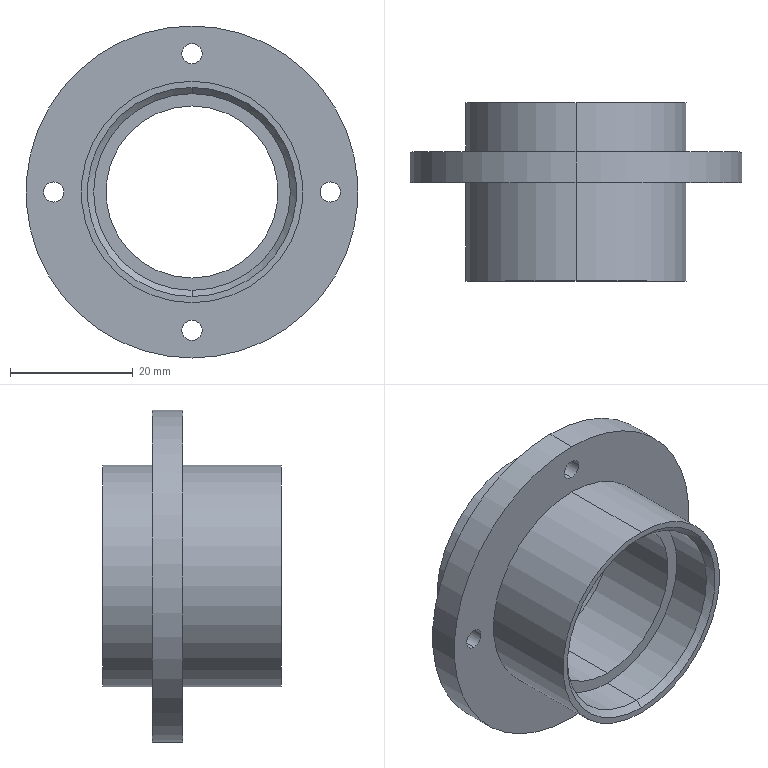Part | SolidWorks | features ICE 5, Chamfer 1, Extrusion 1, HoleWzd 1 | 1 solid | 30 faces | box 54 x 29 x 54 mm | volume 14771 mm3 | cylinder 20 | plane 6 | cone 4 | commonest cylinder face diameters 3.3 x8 32 x4 36 x4 28 x2 54 x2
STEP:
#1=CARTESIAN_POINT('',(0.,7.,-16.));
#2=VERTEX_POINT('',#1);
#3=CARTESIAN_POINT('',(0.,7.,16.));
#4=VERTEX_POINT('',#3);
#5=CARTESIAN_POINT('',(0.,7.,0.));
#6=DIRECTION('',(0.,1.,0.));
#7=DIRECTION('',(0.,0.,1.));
#8=AXIS2_PLACEMENT_3D('',#5,#6,#7);
#9=CIRCLE('',#8,16.);
#10=EDGE_CURVE('',#2,#4,#9,.T.);
#11=ORIENTED_EDGE('',*,*,#10,.F.);
#12=CARTESIAN_POINT('',(0.,8.,-17.));
#13=VERTEX_POINT('',#12);
#14=CARTESIAN_POINT('',(0.,8.,-17.));
#15=DIRECTION('',(0.,0.7071,-0.7071));
#16=VECTOR('',#15,1000.);
#17=LINE('',#14,#16);
#18=EDGE_CURVE('',#2,#13,#17,.T.);
#19=ORIENTED_EDGE('',*,*,#18,.T.);
#20=CARTESIAN_POINT('',(0.,8.,17.));
#21=VERTEX_POINT('',#20);
#22=CARTESIAN_POINT('',(0.,8.,0.));
#23=DIRECTION('',(0.,-1.,0.));
#24=DIRECTION('',(0.,0.,1.));
#25=AXIS2_PLACEMENT_3D('',#22,#23,#24);
#26=CIRCLE('',#25,17.);
#27=EDGE_CURVE('',#21,#13,#26,.T.);
#28=ORIENTED_EDGE('',*,*,#27,.F.);
#29=CARTESIAN_POINT('',(0.,8.,17.));
#30=DIRECTION('',(0.,0.7071,0.7071));
#31=VECTOR('',#30,1000.);
#32=LINE('',#29,#31);
#33=EDGE_CURVE('',#4,#21,#32,.T.);
#34=ORIENTED_EDGE('',*,*,#33,.F.);
#35=EDGE_LOOP('',(#11,#19,#28,#34));
#36=FACE_OUTER_BOUND('',#35,.T.);
#37=CARTESIAN_POINT('',(0.,8.,0.));
#38=DIRECTION('',(0.,1.,0.));
#39=DIRECTION('',(0.,0.,1.));
#40=AXIS2_PLACEMENT_3D('',#37,#38,#39);
#41=CONICAL_SURFACE('',#40,17.,0.7854);
#42=ADVANCED_FACE('',(#36),#41,.F.);
#43=CARTESIAN_POINT('',(0.,-20.,16.));
#44=VERTEX_POINT('',#43);
#45=CARTESIAN_POINT('',(0.,-20.,-16.));
#46=VERTEX_POINT('',#45);
#47=CARTESIAN_POINT('',(0.,-20.,0.));
#48=DIRECTION('',(0.,-1.,0.));
#49=DIRECTION('',(0.,0.,-1.));
#50=AXIS2_PLACEMENT_3D('',#47,#48,#49);
#51=CIRCLE('',#50,16.);
#52=EDGE_CURVE('',#44,#46,#51,.T.);
#53=ORIENTED_EDGE('',*,*,#52,.F.);
#54=CARTESIAN_POINT('',(0.,-21.,17.));
#55=VERTEX_POINT('',#54);
#56=CARTESIAN_POINT('',(0.,-20.,16.));
#57=DIRECTION('',(0.,-0.7071,0.7071));
#58=VECTOR('',#57,1000.);
#59=LINE('',#56,#58);
#60=EDGE_CURVE('',#44,#55,#59,.T.);
#61=ORIENTED_EDGE('',*,*,#60,.T.);
#62=CARTESIAN_POINT('',(0.,-21.,-17.));
#63=VERTEX_POINT('',#62);
#64=CARTESIAN_POINT('',(0.,-21.,0.));
#65=DIRECTION('',(0.,1.,0.));
#66=DIRECTION('',(0.,0.,-1.));
#67=AXIS2_PLACEMENT_3D('',#64,#65,#66);
#68=CIRCLE('',#67,17.);
#69=EDGE_CURVE('',#63,#55,#68,.T.);
#70=ORIENTED_EDGE('',*,*,#69,.F.);
#71=CARTESIAN_POINT('',(0.,-20.,-16.));
#72=DIRECTION('',(0.,-0.7071,-0.7071));
#73=VECTOR('',#72,1000.);
#74=LINE('',#71,#73);
#75=EDGE_CURVE('',#46,#63,#74,.T.);
#76=ORIENTED_EDGE('',*,*,#75,.F.);
#77=EDGE_LOOP('',(#53,#61,#70,#76));
#78=FACE_OUTER_BOUND('',#77,.T.);
#79=CARTESIAN_POINT('',(0.,-20.,0.));
#80=DIRECTION('',(0.,-1.,0.));
#81=DIRECTION('',(0.,0.,-1.));
#82=AXIS2_PLACEMENT_3D('',#79,#80,#81);
#83=CONICAL_SURFACE('',#82,16.,0.7854);
#84=ADVANCED_FACE('',(#78),#83,.F.);
#85=CARTESIAN_POINT('',(-22.5,-5.,1.65));
#86=VERTEX_POINT('',#85);
#87=CARTESIAN_POINT('',(-22.5,-5.,-1.65));
#88=VERTEX_POINT('',#87);
#89=CARTESIAN_POINT('',(-22.5,-5.,0.));
#90=DIRECTION('',(0.,-1.,0.));
#91=DIRECTION('',(0.,0.,-1.));
#92=AXIS2_PLACEMENT_3D('',#89,#90,#91);
#93=CIRCLE('',#92,1.65);
#94=EDGE_CURVE('',#86,#88,#93,.T.);
#95=ORIENTED_EDGE('',*,*,#94,.T.);
#96=CARTESIAN_POINT('',(-22.5,0.,-1.65));
#97=VERTEX_POINT('',#96);
#98=CARTESIAN_POINT('',(-22.5,0.,-1.65));
#99=DIRECTION('',(0.,1.,0.));
#100=VECTOR('',#99,1000.);
#101=LINE('',#98,#100);
#102=EDGE_CURVE('',#88,#97,#101,.T.);
#103=ORIENTED_EDGE('',*,*,#102,.T.);
#104=CARTESIAN_POINT('',(-22.5,0.,1.65));
#105=VERTEX_POINT('',#104);
#106=CARTESIAN_POINT('',(-22.5,0.,0.));
#107=DIRECTION('',(0.,1.,0.));
#108=DIRECTION('',(0.,0.,1.));
#109=AXIS2_PLACEMENT_3D('',#106,#107,#108);
#110=CIRCLE('',#109,1.65);
#111=EDGE_CURVE('',#97,#105,#110,.T.);
#112=ORIENTED_EDGE('',*,*,#111,.T.);
#113=CARTESIAN_POINT('',(-22.5,0.,1.65));
#114=DIRECTION('',(0.,1.,0.));
#115=VECTOR('',#114,1000.);
#116=LINE('',#113,#115);
#117=EDGE_CURVE('',#86,#105,#116,.T.);
#118=ORIENTED_EDGE('',*,*,#117,.F.);
#119=EDGE_LOOP('',(#95,#103,#112,#118));
#120=FACE_OUTER_BOUND('',#119,.T.);
#121=CARTESIAN_POINT('',(-22.5,0.,0.));
#122=DIRECTION('',(0.,1.,0.));
#123=DIRECTION('',(0.,0.,1.));
#124=AXIS2_PLACEMENT_3D('',#121,#122,#123);
#125=CYLINDRICAL_SURFACE('',#124,1.65);
#126=ADVANCED_FACE('',(#120),#125,.F.);
#127=CARTESIAN_POINT('',(0.,-5.,-20.85));
#128=VERTEX_POINT('',#127);
#129=CARTESIAN_POINT('',(0.,-5.,-24.15));
#130=VERTEX_POINT('',#129);
#131=CARTESIAN_POINT('',(0.,-5.,-22.5));
#132=DIRECTION('',(0.,-1.,0.));
#133=DIRECTION('',(0.,0.,-1.));
#134=AXIS2_PLACEMENT_3D('',#131,#132,#133);
#135=CIRCLE('',#134,1.65);
#136=EDGE_CURVE('',#128,#130,#135,.T.);
#137=ORIENTED_EDGE('',*,*,#136,.T.);
#138=CARTESIAN_POINT('',(0.,0.,-24.15));
#139=VERTEX_POINT('',#138);
#140=CARTESIAN_POINT('',(0.,0.,-24.15));
#141=DIRECTION('',(0.,1.,0.));
#142=VECTOR('',#141,1000.);
#143=LINE('',#140,#142);
#144=EDGE_CURVE('',#130,#139,#143,.T.);
#145=ORIENTED_EDGE('',*,*,#144,.T.);
#146=CARTESIAN_POINT('',(0.,0.,-20.85));
#147=VERTEX_POINT('',#146);
#148=CARTESIAN_POINT('',(0.,0.,-22.5));
#149=DIRECTION('',(0.,1.,0.));
#150=DIRECTION('',(0.,0.,1.));
#151=AXIS2_PLACEMENT_3D('',#148,#149,#150);
#152=CIRCLE('',#151,1.65);
#153=EDGE_CURVE('',#139,#147,#152,.T.);
#154=ORIENTED_EDGE('',*,*,#153,.T.);
#155=CARTESIAN_POINT('',(0.,0.,-20.85));
#156=DIRECTION('',(0.,1.,0.));
#157=VECTOR('',#156,1000.);
#158=LINE('',#155,#157);
#159=EDGE_CURVE('',#128,#147,#158,.T.);
#160=ORIENTED_EDGE('',*,*,#159,.F.);
#161=EDGE_LOOP('',(#137,#145,#154,#160));
#162=FACE_OUTER_BOUND('',#161,.T.);
#163=CARTESIAN_POINT('',(0.,0.,-22.5));
#164=DIRECTION('',(0.,1.,0.));
#165=DIRECTION('',(0.,0.,1.));
#166=AXIS2_PLACEMENT_3D('',#163,#164,#165);
#167=CYLINDRICAL_SURFACE('',#166,1.65);
#168=ADVANCED_FACE('',(#162),#167,.F.);
#169=CARTESIAN_POINT('',(22.5,-5.,1.65));
#170=VERTEX_POINT('',#169);
#171=CARTESIAN_POINT('',(22.5,-5.,-1.65));
#172=VERTEX_POINT('',#171);
#173=CARTESIAN_POINT('',(22.5,-5.,0.));
#174=DIRECTION('',(0.,-1.,0.));
#175=DIRECTION('',(0.,0.,-1.));
#176=AXIS2_PLACEMENT_3D('',#173,#174,#175);
#177=CIRCLE('',#176,1.65);
#178=EDGE_CURVE('',#170,#172,#177,.T.);
#179=ORIENTED_EDGE('',*,*,#178,.T.);
#180=CARTESIAN_POINT('',(22.5,0.,-1.65));
#181=VERTEX_POINT('',#180);
#182=CARTESIAN_POINT('',(22.5,0.,-1.65));
#183=DIRECTION('',(0.,1.,0.));
#184=VECTOR('',#183,1000.);
#185=LINE('',#182,#184);
#186=EDGE_CURVE('',#172,#181,#185,.T.);
#187=ORIENTED_EDGE('',*,*,#186,.T.);
#188=CARTESIAN_POINT('',(22.5,0.,1.65));
#189=VERTEX_POINT('',#188);
#190=CARTESIAN_POINT('',(22.5,0.,0.));
#191=DIRECTION('',(0.,1.,0.));
#192=DIRECTION('',(0.,0.,1.));
#193=AXIS2_PLACEMENT_3D('',#190,#191,#192);
#194=CIRCLE('',#193,1.65);
#195=EDGE_CURVE('',#181,#189,#194,.T.);
#196=ORIENTED_EDGE('',*,*,#195,.T.);
#197=CARTESIAN_POINT('',(22.5,0.,1.65));
#198=DIRECTION('',(0.,1.,0.));
#199=VECTOR('',#198,1000.);
#200=LINE('',#197,#199);
#201=EDGE_CURVE('',#170,#189,#200,.T.);
#202=ORIENTED_EDGE('',*,*,#201,.F.);
#203=EDGE_LOOP('',(#179,#187,#196,#202));
#204=FACE_OUTER_BOUND('',#203,.T.);
#205=CARTESIAN_POINT('',(22.5,0.,0.));
#206=DIRECTION('',(0.,1.,0.));
#207=DIRECTION('',(0.,0.,1.));
#208=AXIS2_PLACEMENT_3D('',#205,#206,#207);
#209=CYLINDRICAL_SURFACE('',#208,1.65);
#210=ADVANCED_FACE('',(#204),#209,.F.);
#211=CARTESIAN_POINT('',(0.,-5.,24.15));
#212=VERTEX_POINT('',#211);
#213=CARTESIAN_POINT('',(0.,-5.,20.85));
#214=VERTEX_POINT('',#213);
#215=CARTESIAN_POINT('',(0.,-5.,22.5));
#216=DIRECTION('',(0.,-1.,0.));
#217=DIRECTION('',(0.,0.,-1.));
#218=AXIS2_PLACEMENT_3D('',#215,#216,#217);
#219=CIRCLE('',#218,1.65);
#220=EDGE_CURVE('',#212,#214,#219,.T.);
#221=ORIENTED_EDGE('',*,*,#220,.T.);
#222=CARTESIAN_POINT('',(0.,0.,20.85));
#223=VERTEX_POINT('',#222);
#224=CARTESIAN_POINT('',(0.,0.,20.85));
#225=DIRECTION('',(0.,1.,0.));
#226=VECTOR('',#225,1000.);
#227=LINE('',#224,#226);
#228=EDGE_CURVE('',#214,#223,#227,.T.);
#229=ORIENTED_EDGE('',*,*,#228,.T.);
#230=CARTESIAN_POINT('',(0.,0.,24.15));
#231=VERTEX_POINT('',#230);
#232=CARTESIAN_POINT('',(0.,0.,22.5));
#233=DIRECTION('',(0.,1.,0.));
#234=DIRECTION('',(0.,0.,1.));
#235=AXIS2_PLACEMENT_3D('',#232,#233,#234);
#236=CIRCLE('',#235,1.65);
#237=EDGE_CURVE('',#223,#231,#236,.T.);
#238=ORIENTED_EDGE('',*,*,#237,.T.);
#239=CARTESIAN_POINT('',(0.,0.,24.15));
#240=DIRECTION('',(0.,1.,0.));
#241=VECTOR('',#240,1000.);
#242=LINE('',#239,#241);
#243=EDGE_CURVE('',#212,#231,#242,.T.);
#244=ORIENTED_EDGE('',*,*,#243,.F.);
#245=EDGE_LOOP('',(#221,#229,#238,#244));
#246=FACE_OUTER_BOUND('',#245,.T.);
#247=CARTESIAN_POINT('',(0.,0.,22.5));
#248=DIRECTION('',(0.,1.,0.));
#249=DIRECTION('',(0.,0.,1.));
#250=AXIS2_PLACEMENT_3D('',#247,#248,#249);
#251=CYLINDRICAL_SURFACE('',#250,1.65);
#252=ADVANCED_FACE('',(#246),#251,.F.);
#253=CARTESIAN_POINT('',(0.,-13.2,14.));
#254=VERTEX_POINT('',#253);
#255=CARTESIAN_POINT('',(0.,-13.2,-14.));
#256=VERTEX_POINT('',#255);
#257=CARTESIAN_POINT('',(0.,-13.2,0.));
#258=DIRECTION('',(0.,-1.,0.));
#259=DIRECTION('',(0.,0.,-1.));
#260=AXIS2_PLACEMENT_3D('',#257,#258,#259);
#261=CIRCLE('',#260,14.);
#262=EDGE_CURVE('',#254,#256,#261,.T.);
#263=ORIENTED_EDGE('',*,*,#262,.T.);
#264=CARTESIAN_POINT('',(0.,0.,-14.));
#265=VERTEX_POINT('',#264);
#266=CARTESIAN_POINT('',(0.,-21.,-14.));
#267=DIRECTION('',(0.,1.,0.));
#268=VECTOR('',#267,1000.);
#269=LINE('',#266,#268);
#270=EDGE_CURVE('',#256,#265,#269,.T.);
#271=ORIENTED_EDGE('',*,*,#270,.T.);
#272=CARTESIAN_POINT('',(0.,0.,14.));
#273=VERTEX_POINT('',#272);
#274=CARTESIAN_POINT('',(0.,0.,0.));
#275=DIRECTION('',(0.,1.,0.));
#276=DIRECTION('',(0.,0.,1.));
#277=AXIS2_PLACEMENT_3D('',#274,#275,#276);
#278=CIRCLE('',#277,14.);
#279=EDGE_CURVE('',#265,#273,#278,.T.);
#280=ORIENTED_EDGE('',*,*,#279,.T.);
#281=CARTESIAN_POINT('',(0.,-21.,14.));
#282=DIRECTION('',(0.,1.,0.));
#283=VECTOR('',#282,1000.);
#284=LINE('',#281,#283);
#285=EDGE_CURVE('',#254,#273,#284,.T.);
#286=ORIENTED_EDGE('',*,*,#285,.F.);
#287=EDGE_LOOP('',(#263,#271,#280,#286));
#288=FACE_OUTER_BOUND('',#287,.T.);
#289=CARTESIAN_POINT('',(0.,-21.,0.));
#290=DIRECTION('',(0.,1.,0.));
#291=DIRECTION('',(0.,0.,1.));
#292=AXIS2_PLACEMENT_3D('',#289,#290,#291);
#293=CYLINDRICAL_SURFACE('',#292,14.);
#294=ADVANCED_FACE('',(#288),#293,.F.);
#295=CARTESIAN_POINT('',(0.,-13.2,16.));
#296=VERTEX_POINT('',#295);
#297=CARTESIAN_POINT('',(0.,-13.2,-16.));
#298=VERTEX_POINT('',#297);
#299=CARTESIAN_POINT('',(0.,-13.2,0.));
#300=DIRECTION('',(0.,-1.,0.));
#301=DIRECTION('',(0.,0.,-1.));
#302=AXIS2_PLACEMENT_3D('',#299,#300,#301);
#303=CIRCLE('',#302,16.);
#304=EDGE_CURVE('',#296,#298,#303,.T.);
#305=ORIENTED_EDGE('',*,*,#304,.F.);
#306=CARTESIAN_POINT('',(0.,-13.2,16.));
#307=DIRECTION('',(0.,-1.,0.));
#308=VECTOR('',#307,1000.);
#309=LINE('',#306,#308);
#310=EDGE_CURVE('',#296,#44,#309,.T.);
#311=ORIENTED_EDGE('',*,*,#310,.T.);
#312=ORIENTED_EDGE('',*,*,#52,.T.);
#313=CARTESIAN_POINT('',(0.,-13.2,-16.));
#314=DIRECTION('',(0.,-1.,0.));
#315=VECTOR('',#314,1000.);
#316=LINE('',#313,#315);
#317=EDGE_CURVE('',#298,#46,#316,.T.);
#318=ORIENTED_EDGE('',*,*,#317,.F.);
#319=EDGE_LOOP('',(#305,#311,#312,#318));
#320=FACE_OUTER_BOUND('',#319,.T.);
#321=CARTESIAN_POINT('',(0.,-13.2,0.));
#322=DIRECTION('',(0.,-1.,0.));
#323=DIRECTION('',(0.,0.,-1.));
#324=AXIS2_PLACEMENT_3D('',#321,#322,#323);
#325=CYLINDRICAL_SURFACE('',#324,16.);
#326=ADVANCED_FACE('',(#320),#325,.F.);
#327=CARTESIAN_POINT('',(0.,-21.,-18.));
#328=VERTEX_POINT('',#327);
#329=CARTESIAN_POINT('',(0.,-21.,18.));
#330=VERTEX_POINT('',#329);
#331=CARTESIAN_POINT('',(0.,-21.,0.));
#332=DIRECTION('',(0.,-1.,0.));
#333=DIRECTION('',(0.,0.,-1.));
#334=AXIS2_PLACEMENT_3D('',#331,#332,#333);
#335=CIRCLE('',#334,18.);
#336=EDGE_CURVE('',#328,#330,#335,.T.);
#337=ORIENTED_EDGE('',*,*,#336,.F.);
#338=CARTESIAN_POINT('',(0.,-5.,-18.));
#339=VERTEX_POINT('',#338);
#340=CARTESIAN_POINT('',(0.,-21.,-18.));
#341=DIRECTION('',(0.,1.,0.));
#342=VECTOR('',#341,1000.);
#343=LINE('',#340,#342);
#344=EDGE_CURVE('',#328,#339,#343,.T.);
#345=ORIENTED_EDGE('',*,*,#344,.T.);
#346=CARTESIAN_POINT('',(0.,-5.,18.));
#347=VERTEX_POINT('',#346);
#348=CARTESIAN_POINT('',(0.,-5.,0.));
#349=DIRECTION('',(0.,-1.,0.));
#350=DIRECTION('',(0.,0.,-1.));
#351=AXIS2_PLACEMENT_3D('',#348,#349,#350);
#352=CIRCLE('',#351,18.);
#353=EDGE_CURVE('',#339,#347,#352,.T.);
#354=ORIENTED_EDGE('',*,*,#353,.T.);
#355=CARTESIAN_POINT('',(0.,-21.,18.));
#356=DIRECTION('',(0.,1.,0.));
#357=VECTOR('',#356,1000.);
#358=LINE('',#355,#357);
#359=EDGE_CURVE('',#330,#347,#358,.T.);
#360=ORIENTED_EDGE('',*,*,#359,.F.);
#361=EDGE_LOOP('',(#337,#345,#354,#360));
#362=FACE_OUTER_BOUND('',#361,.T.);
#363=CARTESIAN_POINT('',(0.,-21.,0.));
#364=DIRECTION('',(0.,1.,0.));
#365=DIRECTION('',(0.,0.,1.));
#366=AXIS2_PLACEMENT_3D('',#363,#364,#365);
#367=CYLINDRICAL_SURFACE('',#366,18.);
#368=ADVANCED_FACE('',(#362),#367,.T.);
#369=CARTESIAN_POINT('',(0.,-5.,-27.));
#370=VERTEX_POINT('',#369);
#371=CARTESIAN_POINT('',(0.,-5.,27.));
#372=VERTEX_POINT('',#371);
#373=CARTESIAN_POINT('',(0.,-5.,0.));
#374=DIRECTION('',(0.,-1.,0.));
#375=DIRECTION('',(0.,0.,-1.));
#376=AXIS2_PLACEMENT_3D('',#373,#374,#375);
#377=CIRCLE('',#376,27.);
#378=EDGE_CURVE('',#370,#372,#377,.T.);
#379=ORIENTED_EDGE('',*,*,#378,.F.);
#380=CARTESIAN_POINT('',(0.,0.,-27.));
#381=VERTEX_POINT('',#380);
#382=CARTESIAN_POINT('',(0.,-5.,-27.));
#383=DIRECTION('',(0.,1.,0.));
#384=VECTOR('',#383,1000.);
#385=LINE('',#382,#384);
#386=EDGE_CURVE('',#370,#381,#385,.T.);
#387=ORIENTED_EDGE('',*,*,#386,.T.);
#388=CARTESIAN_POINT('',(0.,0.,27.));
#389=VERTEX_POINT('',#388);
#390=CARTESIAN_POINT('',(0.,0.,0.));
#391=DIRECTION('',(0.,-1.,0.));
#392=DIRECTION('',(0.,0.,-1.));
#393=AXIS2_PLACEMENT_3D('',#390,#391,#392);
#394=CIRCLE('',#393,27.);
#395=EDGE_CURVE('',#381,#389,#394,.T.);
#396=ORIENTED_EDGE('',*,*,#395,.T.);
#397=CARTESIAN_POINT('',(0.,-5.,27.));
#398=DIRECTION('',(0.,1.,0.));
#399=VECTOR('',#398,1000.);
#400=LINE('',#397,#399);
#401=EDGE_CURVE('',#372,#389,#400,.T.);
#402=ORIENTED_EDGE('',*,*,#401,.F.);
#403=EDGE_LOOP('',(#379,#387,#396,#402));
#404=FACE_OUTER_BOUND('',#403,.T.);
#405=CARTESIAN_POINT('',(0.,-5.,0.));
#406=DIRECTION('',(0.,1.,0.));
#407=DIRECTION('',(0.,0.,1.));
#408=AXIS2_PLACEMENT_3D('',#405,#406,#407);
#409=CYLINDRICAL_SURFACE('',#408,27.);
#410=ADVANCED_FACE('',(#404),#409,.T.);
#411=ORIENTED_EDGE('',*,*,#10,.T.);
#412=CARTESIAN_POINT('',(0.,0.,16.));
#413=VERTEX_POINT('',#412);
#414=CARTESIAN_POINT('',(0.,8.001,16.));
#415=DIRECTION('',(0.,-1.,0.));
#416=VECTOR('',#415,1000.);
#417=LINE('',#414,#416);
#418=EDGE_CURVE('',#4,#413,#417,.T.);
#419=ORIENTED_EDGE('',*,*,#418,.T.);
#420=CARTESIAN_POINT('',(0.,0.,-16.));
#421=VERTEX_POINT('',#420);
#422=CARTESIAN_POINT('',(0.,0.,0.));
#423=DIRECTION('',(0.,1.,0.));
#424=DIRECTION('',(0.,0.,-1.));
#425=AXIS2_PLACEMENT_3D('',#422,#423,#424);
#426=CIRCLE('',#425,16.);
#427=EDGE_CURVE('',#421,#413,#426,.T.);
#428=ORIENTED_EDGE('',*,*,#427,.F.);
#429=CARTESIAN_POINT('',(0.,8.001,-16.));
#430=DIRECTION('',(0.,-1.,0.));
#431=VECTOR('',#430,1000.);
#432=LINE('',#429,#431);
#433=EDGE_CURVE('',#2,#421,#432,.T.);
#434=ORIENTED_EDGE('',*,*,#433,.F.);
#435=EDGE_LOOP('',(#411,#419,#428,#434));
#436=FACE_OUTER_BOUND('',#435,.T.);
#437=CARTESIAN_POINT('',(0.,8.001,0.));
#438=DIRECTION('',(0.,-1.,0.));
#439=DIRECTION('',(0.,0.,-1.));
#440=AXIS2_PLACEMENT_3D('',#437,#438,#439);
#441=CYLINDRICAL_SURFACE('',#440,16.);
#442=ADVANCED_FACE('',(#436),#441,.F.);
#443=CARTESIAN_POINT('',(0.,8.,18.));
#444=VERTEX_POINT('',#443);
#445=CARTESIAN_POINT('',(0.,8.,-18.));
#446=VERTEX_POINT('',#445);
#447=CARTESIAN_POINT('',(0.,8.,0.));
#448=DIRECTION('',(0.,1.,0.));
#449=DIRECTION('',(0.,0.,1.));
#450=AXIS2_PLACEMENT_3D('',#447,#448,#449);
#451=CIRCLE('',#450,18.);
#452=EDGE_CURVE('',#444,#446,#451,.T.);
#453=ORIENTED_EDGE('',*,*,#452,.F.);
#454=CARTESIAN_POINT('',(0.,0.,18.));
#455=VERTEX_POINT('',#454);
#456=CARTESIAN_POINT('',(0.,8.,18.));
#457=DIRECTION('',(0.,-1.,0.));
#458=VECTOR('',#457,1000.);
#459=LINE('',#456,#458);
#460=EDGE_CURVE('',#444,#455,#459,.T.);
#461=ORIENTED_EDGE('',*,*,#460,.T.);
#462=CARTESIAN_POINT('',(0.,0.,-18.));
#463=VERTEX_POINT('',#462);
#464=CARTESIAN_POINT('',(0.,0.,0.));
#465=DIRECTION('',(0.,-1.,0.));
#466=DIRECTION('',(0.,0.,-1.));
#467=AXIS2_PLACEMENT_3D('',#464,#465,#466);
#468=CIRCLE('',#467,18.);
#469=EDGE_CURVE('',#463,#455,#468,.T.);
#470=ORIENTED_EDGE('',*,*,#469,.F.);
#471=CARTESIAN_POINT('',(0.,8.,-18.));
#472=DIRECTION('',(0.,-1.,0.));
#473=VECTOR('',#472,1000.);
#474=LINE('',#471,#473);
#475=EDGE_CURVE('',#446,#463,#474,.T.);
#476=ORIENTED_EDGE('',*,*,#475,.F.);
#477=EDGE_LOOP('',(#453,#461,#470,#476));
#478=FACE_OUTER_BOUND('',#477,.T.);
#479=CARTESIAN_POINT('',(0.,8.,0.));
#480=DIRECTION('',(0.,-1.,0.));
#481=DIRECTION('',(0.,0.,-1.));
#482=AXIS2_PLACEMENT_3D('',#479,#480,#481);
#483=CYLINDRICAL_SURFACE('',#482,18.);
#484=ADVANCED_FACE('',(#478),#483,.T.);
#485=ORIENTED_EDGE('',*,*,#460,.F.);
#486=CARTESIAN_POINT('',(0.,8.,0.));
#487=DIRECTION('',(0.,1.,0.));
#488=DIRECTION('',(0.,0.,1.));
#489=AXIS2_PLACEMENT_3D('',#486,#487,#488);
#490=CIRCLE('',#489,18.);
#491=EDGE_CURVE('',#446,#444,#490,.T.);
#492=ORIENTED_EDGE('',*,*,#491,.F.);
#493=ORIENTED_EDGE('',*,*,#475,.T.);
#494=CARTESIAN_POINT('',(0.,0.,0.));
#495=DIRECTION('',(0.,-1.,0.));
#496=DIRECTION('',(0.,0.,-1.));
#497=AXIS2_PLACEMENT_3D('',#494,#495,#496);
#498=CIRCLE('',#497,18.);
#499=EDGE_CURVE('',#455,#463,#498,.T.);
#500=ORIENTED_EDGE('',*,*,#499,.F.);
#501=EDGE_LOOP('',(#485,#492,#493,#500));
#502=FACE_OUTER_BOUND('',#501,.T.);
#503=CARTESIAN_POINT('',(0.,8.,0.));
#504=DIRECTION('',(0.,-1.,0.));
#505=DIRECTION('',(0.,0.,-1.));
#506=AXIS2_PLACEMENT_3D('',#503,#504,#505);
#507=CYLINDRICAL_SURFACE('',#506,18.);
#508=ADVANCED_FACE('',(#502),#507,.T.);
#509=ORIENTED_EDGE('',*,*,#27,.T.);
#510=CARTESIAN_POINT('',(0.,8.,0.));
#511=DIRECTION('',(0.,-1.,0.));
#512=DIRECTION('',(0.,0.,1.));
#513=AXIS2_PLACEMENT_3D('',#510,#511,#512);
#514=CIRCLE('',#513,17.);
#515=EDGE_CURVE('',#13,#21,#514,.T.);
#516=ORIENTED_EDGE('',*,*,#515,.T.);
#517=EDGE_LOOP('',(#509,#516));
#518=FACE_BOUND('',#517,.T.);
#519=ORIENTED_EDGE('',*,*,#491,.T.);
#520=ORIENTED_EDGE('',*,*,#452,.T.);
#521=EDGE_LOOP('',(#519,#520));
#522=FACE_OUTER_BOUND('',#521,.T.);
#523=CARTESIAN_POINT('',(0.,8.,0.));
#524=DIRECTION('',(0.,1.,0.));
#525=DIRECTION('',(0.,0.,1.));
#526=AXIS2_PLACEMENT_3D('',#523,#524,#525);
#527=PLANE('',#526);
#528=ADVANCED_FACE('',(#518,#522),#527,.T.);
#529=ORIENTED_EDGE('',*,*,#418,.F.);
#530=CARTESIAN_POINT('',(0.,7.,0.));
#531=DIRECTION('',(0.,1.,0.));
#532=DIRECTION('',(0.,0.,1.));
#533=AXIS2_PLACEMENT_3D('',#530,#531,#532);
#534=CIRCLE('',#533,16.);
#535=EDGE_CURVE('',#4,#2,#534,.T.);
#536=ORIENTED_EDGE('',*,*,#535,.T.);
#537=ORIENTED_EDGE('',*,*,#433,.T.);
#538=CARTESIAN_POINT('',(0.,0.,0.));
#539=DIRECTION('',(0.,1.,0.));
#540=DIRECTION('',(0.,0.,-1.));
#541=AXIS2_PLACEMENT_3D('',#538,#539,#540);
#542=CIRCLE('',#541,16.);
#543=EDGE_CURVE('',#413,#421,#542,.T.);
#544=ORIENTED_EDGE('',*,*,#543,.F.);
#545=EDGE_LOOP('',(#529,#536,#537,#544));
#546=FACE_OUTER_BOUND('',#545,.T.);
#547=CARTESIAN_POINT('',(0.,8.001,0.));
#548=DIRECTION('',(0.,-1.,0.));
#549=DIRECTION('',(0.,0.,-1.));
#550=AXIS2_PLACEMENT_3D('',#547,#548,#549);
#551=CYLINDRICAL_SURFACE('',#550,16.);
#552=ADVANCED_FACE('',(#546),#551,.F.);
#553=CARTESIAN_POINT('',(0.,0.,0.));
#554=DIRECTION('',(0.,1.,0.));
#555=DIRECTION('',(0.,0.,1.));
#556=AXIS2_PLACEMENT_3D('',#553,#554,#555);
#557=CIRCLE('',#556,14.);
#558=EDGE_CURVE('',#273,#265,#557,.T.);
#559=ORIENTED_EDGE('',*,*,#558,.F.);
#560=ORIENTED_EDGE('',*,*,#279,.F.);
#561=EDGE_LOOP('',(#559,#560));
#562=FACE_BOUND('',#561,.T.);
#563=ORIENTED_EDGE('',*,*,#427,.T.);
#564=ORIENTED_EDGE('',*,*,#543,.T.);
#565=EDGE_LOOP('',(#563,#564));
#566=FACE_OUTER_BOUND('',#565,.T.);
#567=CARTESIAN_POINT('',(0.,0.,0.));
#568=DIRECTION('',(0.,-1.,0.));
#569=DIRECTION('',(0.,0.,-1.));
#570=AXIS2_PLACEMENT_3D('',#567,#568,#569);
#571=PLANE('',#570);
#572=ADVANCED_FACE('',(#562,#566),#571,.F.);
#573=CARTESIAN_POINT('',(-22.5,0.,0.));
#574=DIRECTION('',(0.,1.,0.));
#575=DIRECTION('',(0.,0.,1.));
#576=AXIS2_PLACEMENT_3D('',#573,#574,#575);
#577=CIRCLE('',#576,1.65);
#578=EDGE_CURVE('',#105,#97,#577,.T.);
#579=ORIENTED_EDGE('',*,*,#578,.F.);
#580=ORIENTED_EDGE('',*,*,#111,.F.);
#581=EDGE_LOOP('',(#579,#580));
#582=FACE_BOUND('',#581,.T.);
#583=CARTESIAN_POINT('',(0.,0.,-22.5));
#584=DIRECTION('',(0.,1.,0.));
#585=DIRECTION('',(0.,0.,1.));
#586=AXIS2_PLACEMENT_3D('',#583,#584,#585);
#587=CIRCLE('',#586,1.65);
#588=EDGE_CURVE('',#147,#139,#587,.T.);
#589=ORIENTED_EDGE('',*,*,#588,.F.);
#590=ORIENTED_EDGE('',*,*,#153,.F.);
#591=EDGE_LOOP('',(#589,#590));
#592=FACE_BOUND('',#591,.T.);
#593=CARTESIAN_POINT('',(22.5,0.,0.));
#594=DIRECTION('',(0.,1.,0.));
#595=DIRECTION('',(0.,0.,1.));
#596=AXIS2_PLACEMENT_3D('',#593,#594,#595);
#597=CIRCLE('',#596,1.65);
#598=EDGE_CURVE('',#189,#181,#597,.T.);
#599=ORIENTED_EDGE('',*,*,#598,.F.);
#600=ORIENTED_EDGE('',*,*,#195,.F.);
#601=EDGE_LOOP('',(#599,#600));
#602=FACE_BOUND('',#601,.T.);
#603=CARTESIAN_POINT('',(0.,0.,22.5));
#604=DIRECTION('',(0.,1.,0.));
#605=DIRECTION('',(0.,0.,1.));
#606=AXIS2_PLACEMENT_3D('',#603,#604,#605);
#607=CIRCLE('',#606,1.65);
#608=EDGE_CURVE('',#231,#223,#607,.T.);
#609=ORIENTED_EDGE('',*,*,#608,.F.);
#610=ORIENTED_EDGE('',*,*,#237,.F.);
#611=EDGE_LOOP('',(#609,#610));
#612=FACE_BOUND('',#611,.T.);
#613=CARTESIAN_POINT('',(0.,0.,0.));
#614=DIRECTION('',(0.,-1.,0.));
#615=DIRECTION('',(0.,0.,-1.));
#616=AXIS2_PLACEMENT_3D('',#613,#614,#615);
#617=CIRCLE('',#616,27.);
#618=EDGE_CURVE('',#389,#381,#617,.T.);
#619=ORIENTED_EDGE('',*,*,#618,.F.);
#620=ORIENTED_EDGE('',*,*,#395,.F.);
#621=EDGE_LOOP('',(#619,#620));
#622=FACE_OUTER_BOUND('',#621,.T.);
#623=ORIENTED_EDGE('',*,*,#469,.T.);
#624=ORIENTED_EDGE('',*,*,#499,.T.);
#625=EDGE_LOOP('',(#623,#624));
#626=FACE_BOUND('',#625,.T.);
#627=CARTESIAN_POINT('',(0.,0.,0.));
#628=DIRECTION('',(0.,-1.,0.));
#629=DIRECTION('',(0.,0.,-1.));
#630=AXIS2_PLACEMENT_3D('',#627,#628,#629);
#631=PLANE('',#630);
#632=ADVANCED_FACE('',(#582,#592,#602,#612,#622,#626),#631,.F.);
#633=ORIENTED_EDGE('',*,*,#386,.F.);
#634=CARTESIAN_POINT('',(0.,-5.,0.));
#635=DIRECTION('',(0.,-1.,0.));
#636=DIRECTION('',(0.,0.,-1.));
#637=AXIS2_PLACEMENT_3D('',#634,#635,#636);
#638=CIRCLE('',#637,27.);
#639=EDGE_CURVE('',#372,#370,#638,.T.);
#640=ORIENTED_EDGE('',*,*,#639,.F.);
#641=ORIENTED_EDGE('',*,*,#401,.T.);
#642=ORIENTED_EDGE('',*,*,#618,.T.);
#643=EDGE_LOOP('',(#633,#640,#641,#642));
#644=FACE_OUTER_BOUND('',#643,.T.);
#645=CARTESIAN_POINT('',(0.,-5.,0.));
#646=DIRECTION('',(0.,1.,0.));
#647=DIRECTION('',(0.,0.,1.));
#648=AXIS2_PLACEMENT_3D('',#645,#646,#647);
#649=CYLINDRICAL_SURFACE('',#648,27.);
#650=ADVANCED_FACE('',(#644),#649,.T.);
#651=ORIENTED_EDGE('',*,*,#94,.F.);
#652=CARTESIAN_POINT('',(-22.5,-5.,0.));
#653=DIRECTION('',(0.,-1.,0.));
#654=DIRECTION('',(0.,0.,-1.));
#655=AXIS2_PLACEMENT_3D('',#652,#653,#654);
#656=CIRCLE('',#655,1.65);
#657=EDGE_CURVE('',#88,#86,#656,.T.);
#658=ORIENTED_EDGE('',*,*,#657,.F.);
#659=EDGE_LOOP('',(#651,#658));
#660=FACE_BOUND('',#659,.T.);
#661=ORIENTED_EDGE('',*,*,#136,.F.);
#662=CARTESIAN_POINT('',(0.,-5.,-22.5));
#663=DIRECTION('',(0.,-1.,0.));
#664=DIRECTION('',(0.,0.,-1.));
#665=AXIS2_PLACEMENT_3D('',#662,#663,#664);
#666=CIRCLE('',#665,1.65);
#667=EDGE_CURVE('',#130,#128,#666,.T.);
#668=ORIENTED_EDGE('',*,*,#667,.F.);
#669=EDGE_LOOP('',(#661,#668));
#670=FACE_BOUND('',#669,.T.);
#671=ORIENTED_EDGE('',*,*,#178,.F.);
#672=CARTESIAN_POINT('',(22.5,-5.,0.));
#673=DIRECTION('',(0.,-1.,0.));
#674=DIRECTION('',(0.,0.,-1.));
#675=AXIS2_PLACEMENT_3D('',#672,#673,#674);
#676=CIRCLE('',#675,1.65);
#677=EDGE_CURVE('',#172,#170,#676,.T.);
#678=ORIENTED_EDGE('',*,*,#677,.F.);
#679=EDGE_LOOP('',(#671,#678));
#680=FACE_BOUND('',#679,.T.);
#681=ORIENTED_EDGE('',*,*,#220,.F.);
#682=CARTESIAN_POINT('',(0.,-5.,22.5));
#683=DIRECTION('',(0.,-1.,0.));
#684=DIRECTION('',(0.,0.,-1.));
#685=AXIS2_PLACEMENT_3D('',#682,#683,#684);
#686=CIRCLE('',#685,1.65);
#687=EDGE_CURVE('',#214,#212,#686,.T.);
#688=ORIENTED_EDGE('',*,*,#687,.F.);
#689=EDGE_LOOP('',(#681,#688));
#690=FACE_BOUND('',#689,.T.);
#691=CARTESIAN_POINT('',(0.,-5.,0.));
#692=DIRECTION('',(0.,-1.,0.));
#693=DIRECTION('',(0.,0.,-1.));
#694=AXIS2_PLACEMENT_3D('',#691,#692,#693);
#695=CIRCLE('',#694,18.);
#696=EDGE_CURVE('',#347,#339,#695,.T.);
#697=ORIENTED_EDGE('',*,*,#696,.F.);
#698=ORIENTED_EDGE('',*,*,#353,.F.);
#699=EDGE_LOOP('',(#697,#698));
#700=FACE_BOUND('',#699,.T.);
#701=ORIENTED_EDGE('',*,*,#639,.T.);
#702=ORIENTED_EDGE('',*,*,#378,.T.);
#703=EDGE_LOOP('',(#701,#702));
#704=FACE_OUTER_BOUND('',#703,.T.);
#705=CARTESIAN_POINT('',(0.,-5.,0.));
#706=DIRECTION('',(0.,-1.,0.));
#707=DIRECTION('',(0.,0.,-1.));
#708=AXIS2_PLACEMENT_3D('',#705,#706,#707);
#709=PLANE('',#708);
#710=ADVANCED_FACE('',(#660,#670,#680,#690,#700,#704),#709,.T.);
#711=ORIENTED_EDGE('',*,*,#344,.F.);
#712=CARTESIAN_POINT('',(0.,-21.,0.));
#713=DIRECTION('',(0.,-1.,0.));
#714=DIRECTION('',(0.,0.,-1.));
#715=AXIS2_PLACEMENT_3D('',#712,#713,#714);
#716=CIRCLE('',#715,18.);
#717=EDGE_CURVE('',#330,#328,#716,.T.);
#718=ORIENTED_EDGE('',*,*,#717,.F.);
#719=ORIENTED_EDGE('',*,*,#359,.T.);
#720=ORIENTED_EDGE('',*,*,#696,.T.);
#721=EDGE_LOOP('',(#711,#718,#719,#720));
#722=FACE_OUTER_BOUND('',#721,.T.);
#723=CARTESIAN_POINT('',(0.,-21.,0.));
#724=DIRECTION('',(0.,1.,0.));
#725=DIRECTION('',(0.,0.,1.));
#726=AXIS2_PLACEMENT_3D('',#723,#724,#725);
#727=CYLINDRICAL_SURFACE('',#726,18.);
#728=ADVANCED_FACE('',(#722),#727,.T.);
#729=ORIENTED_EDGE('',*,*,#69,.T.);
#730=CARTESIAN_POINT('',(0.,-21.,0.));
#731=DIRECTION('',(0.,1.,0.));
#732=DIRECTION('',(0.,0.,-1.));
#733=AXIS2_PLACEMENT_3D('',#730,#731,#732);
#734=CIRCLE('',#733,17.);
#735=EDGE_CURVE('',#55,#63,#734,.T.);
#736=ORIENTED_EDGE('',*,*,#735,.T.);
#737=EDGE_LOOP('',(#729,#736));
#738=FACE_BOUND('',#737,.T.);
#739=ORIENTED_EDGE('',*,*,#717,.T.);
#740=ORIENTED_EDGE('',*,*,#336,.T.);
#741=EDGE_LOOP('',(#739,#740));
#742=FACE_OUTER_BOUND('',#741,.T.);
#743=CARTESIAN_POINT('',(0.,-21.,0.));
#744=DIRECTION('',(0.,-1.,0.));
#745=DIRECTION('',(0.,0.,-1.));
#746=AXIS2_PLACEMENT_3D('',#743,#744,#745);
#747=PLANE('',#746);
#748=ADVANCED_FACE('',(#738,#742),#747,.T.);
#749=ORIENTED_EDGE('',*,*,#310,.F.);
#750=CARTESIAN_POINT('',(0.,-13.2,0.));
#751=DIRECTION('',(0.,-1.,0.));
#752=DIRECTION('',(0.,0.,-1.));
#753=AXIS2_PLACEMENT_3D('',#750,#751,#752);
#754=CIRCLE('',#753,16.);
#755=EDGE_CURVE('',#298,#296,#754,.T.);
#756=ORIENTED_EDGE('',*,*,#755,.F.);
#757=ORIENTED_EDGE('',*,*,#317,.T.);
#758=CARTESIAN_POINT('',(0.,-20.,0.));
#759=DIRECTION('',(0.,-1.,0.));
#760=DIRECTION('',(0.,0.,-1.));
#761=AXIS2_PLACEMENT_3D('',#758,#759,#760);
#762=CIRCLE('',#761,16.);
#763=EDGE_CURVE('',#46,#44,#762,.T.);
#764=ORIENTED_EDGE('',*,*,#763,.T.);
#765=EDGE_LOOP('',(#749,#756,#757,#764));
#766=FACE_OUTER_BOUND('',#765,.T.);
#767=CARTESIAN_POINT('',(0.,-13.2,0.));
#768=DIRECTION('',(0.,-1.,0.));
#769=DIRECTION('',(0.,0.,-1.));
#770=AXIS2_PLACEMENT_3D('',#767,#768,#769);
#771=CYLINDRICAL_SURFACE('',#770,16.);
#772=ADVANCED_FACE('',(#766),#771,.F.);
#773=ORIENTED_EDGE('',*,*,#262,.F.);
#774=CARTESIAN_POINT('',(0.,-13.2,0.));
#775=DIRECTION('',(0.,-1.,0.));
#776=DIRECTION('',(0.,0.,-1.));
#777=AXIS2_PLACEMENT_3D('',#774,#775,#776);
#778=CIRCLE('',#777,14.);
#779=EDGE_CURVE('',#256,#254,#778,.T.);
#780=ORIENTED_EDGE('',*,*,#779,.F.);
#781=EDGE_LOOP('',(#773,#780));
#782=FACE_BOUND('',#781,.T.);
#783=ORIENTED_EDGE('',*,*,#755,.T.);
#784=ORIENTED_EDGE('',*,*,#304,.T.);
#785=EDGE_LOOP('',(#783,#784));
#786=FACE_OUTER_BOUND('',#785,.T.);
#787=CARTESIAN_POINT('',(0.,-13.2,0.));
#788=DIRECTION('',(0.,-1.,0.));
#789=DIRECTION('',(0.,0.,-1.));
#790=AXIS2_PLACEMENT_3D('',#787,#788,#789);
#791=PLANE('',#790);
#792=ADVANCED_FACE('',(#782,#786),#791,.T.);
#793=ORIENTED_EDGE('',*,*,#270,.F.);
#794=ORIENTED_EDGE('',*,*,#779,.T.);
#795=ORIENTED_EDGE('',*,*,#285,.T.);
#796=ORIENTED_EDGE('',*,*,#558,.T.);
#797=EDGE_LOOP('',(#793,#794,#795,#796));
#798=FACE_OUTER_BOUND('',#797,.T.);
#799=CARTESIAN_POINT('',(0.,-21.,0.));
#800=DIRECTION('',(0.,1.,0.));
#801=DIRECTION('',(0.,0.,1.));
#802=AXIS2_PLACEMENT_3D('',#799,#800,#801);
#803=CYLINDRICAL_SURFACE('',#802,14.);
#804=ADVANCED_FACE('',(#798),#803,.F.);
#805=ORIENTED_EDGE('',*,*,#228,.F.);
#806=ORIENTED_EDGE('',*,*,#687,.T.);
#807=ORIENTED_EDGE('',*,*,#243,.T.);
#808=ORIENTED_EDGE('',*,*,#608,.T.);
#809=EDGE_LOOP('',(#805,#806,#807,#808));
#810=FACE_OUTER_BOUND('',#809,.T.);
#811=CARTESIAN_POINT('',(0.,0.,22.5));
#812=DIRECTION('',(0.,1.,0.));
#813=DIRECTION('',(0.,0.,1.));
#814=AXIS2_PLACEMENT_3D('',#811,#812,#813);
#815=CYLINDRICAL_SURFACE('',#814,1.65);
#816=ADVANCED_FACE('',(#810),#815,.F.);
#817=ORIENTED_EDGE('',*,*,#186,.F.);
#818=ORIENTED_EDGE('',*,*,#677,.T.);
#819=ORIENTED_EDGE('',*,*,#201,.T.);
#820=ORIENTED_EDGE('',*,*,#598,.T.);
#821=EDGE_LOOP('',(#817,#818,#819,#820));
#822=FACE_OUTER_BOUND('',#821,.T.);
#823=CARTESIAN_POINT('',(22.5,0.,0.));
#824=DIRECTION('',(0.,1.,0.));
#825=DIRECTION('',(0.,0.,1.));
#826=AXIS2_PLACEMENT_3D('',#823,#824,#825);
#827=CYLINDRICAL_SURFACE('',#826,1.65);
#828=ADVANCED_FACE('',(#822),#827,.F.);
#829=ORIENTED_EDGE('',*,*,#144,.F.);
#830=ORIENTED_EDGE('',*,*,#667,.T.);
#831=ORIENTED_EDGE('',*,*,#159,.T.);
#832=ORIENTED_EDGE('',*,*,#588,.T.);
#833=EDGE_LOOP('',(#829,#830,#831,#832));
#834=FACE_OUTER_BOUND('',#833,.T.);
#835=CARTESIAN_POINT('',(0.,0.,-22.5));
#836=DIRECTION('',(0.,1.,0.));
#837=DIRECTION('',(0.,0.,1.));
#838=AXIS2_PLACEMENT_3D('',#835,#836,#837);
#839=CYLINDRICAL_SURFACE('',#838,1.65);
#840=ADVANCED_FACE('',(#834),#839,.F.);
#841=ORIENTED_EDGE('',*,*,#102,.F.);
#842=ORIENTED_EDGE('',*,*,#657,.T.);
#843=ORIENTED_EDGE('',*,*,#117,.T.);
#844=ORIENTED_EDGE('',*,*,#578,.T.);
#845=EDGE_LOOP('',(#841,#842,#843,#844));
#846=FACE_OUTER_BOUND('',#845,.T.);
#847=CARTESIAN_POINT('',(-22.5,0.,0.));
#848=DIRECTION('',(0.,1.,0.));
#849=DIRECTION('',(0.,0.,1.));
#850=AXIS2_PLACEMENT_3D('',#847,#848,#849);
#851=CYLINDRICAL_SURFACE('',#850,1.65);
#852=ADVANCED_FACE('',(#846),#851,.F.);
#853=ORIENTED_EDGE('',*,*,#60,.F.);
#854=ORIENTED_EDGE('',*,*,#763,.F.);
#855=ORIENTED_EDGE('',*,*,#75,.T.);
#856=ORIENTED_EDGE('',*,*,#735,.F.);
#857=EDGE_LOOP('',(#853,#854,#855,#856));
#858=FACE_OUTER_BOUND('',#857,.T.);
#859=CARTESIAN_POINT('',(0.,-20.,0.));
#860=DIRECTION('',(0.,-1.,0.));
#861=DIRECTION('',(0.,0.,-1.));
#862=AXIS2_PLACEMENT_3D('',#859,#860,#861);
#863=CONICAL_SURFACE('',#862,16.,0.7854);
#864=ADVANCED_FACE('',(#858),#863,.F.);
#865=ORIENTED_EDGE('',*,*,#18,.F.);
#866=ORIENTED_EDGE('',*,*,#535,.F.);
#867=ORIENTED_EDGE('',*,*,#33,.T.);
#868=ORIENTED_EDGE('',*,*,#515,.F.);
#869=EDGE_LOOP('',(#865,#866,#867,#868));
#870=FACE_OUTER_BOUND('',#869,.T.);
#871=CARTESIAN_POINT('',(0.,8.,0.));
#872=DIRECTION('',(0.,1.,0.));
#873=DIRECTION('',(0.,0.,1.));
#874=AXIS2_PLACEMENT_3D('',#871,#872,#873);
#875=CONICAL_SURFACE('',#874,17.,0.7854);
#876=ADVANCED_FACE('',(#870),#875,.F.);
#877=CLOSED_SHELL('',(#42,#84,#126,#168,#210,#252,#294,#326,#368,#410,#442,#484,#508,#528,#552,#572,#632,#650,#710,#728,#748,#772,#792,#804,#816,#828,#840,#852,#864,#876));
#878=MANIFOLD_SOLID_BREP('',#877);
#879=CARTESIAN_POINT('',(0.,0.,0.));
#880=DIRECTION('',(0.,0.,1.));
#881=DIRECTION('',(1.,0.,0.));
#882=AXIS2_PLACEMENT_3D('',#879,#880,#881);
#883=(LENGTH_UNIT()NAMED_UNIT(*)SI_UNIT(.MILLI.,.METRE.));
#884=UNCERTAINTY_MEASURE_WITH_UNIT(LENGTH_MEASURE(0.00001),#883,'','');
#885=(NAMED_UNIT(*)PLANE_ANGLE_UNIT()SI_UNIT($,.RADIAN.));
#886=(NAMED_UNIT(*)SI_UNIT($,.STERADIAN.)SOLID_ANGLE_UNIT());
#887=(GEOMETRIC_REPRESENTATION_CONTEXT(3)GLOBAL_UNCERTAINTY_ASSIGNED_CONTEXT((#884))GLOBAL_UNIT_ASSIGNED_CONTEXT((#883,#885,#886))REPRESENTATION_CONTEXT('',''));
#888=ADVANCED_BREP_SHAPE_REPRESENTATION('',(#878,#882),#887);